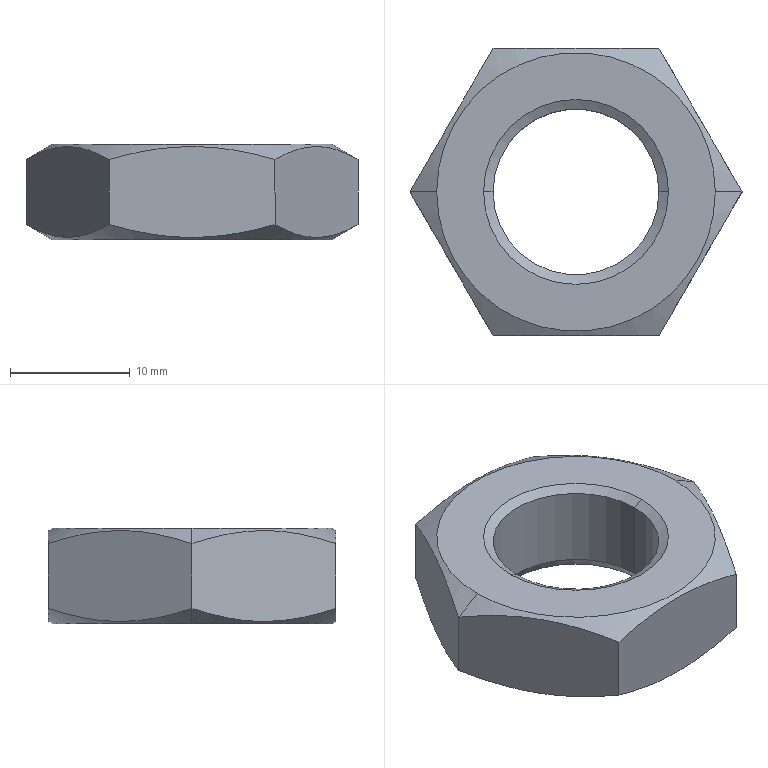Part | SolidWorks | features RevCut 2, Chamfer 1, Extrusion 1, LPattern 1 | 1 solid | 18 faces | box 27.713 x 24 x 8 mm | volume 2715 mm3 | cone 8 | plane 8 | cylinder 2 | commonest cylinder face diameters 13.835 x2
STEP:
#1=CARTESIAN_POINT('',(-6.918,0.,-0.4619));
#2=VERTEX_POINT('',#1);
#3=CARTESIAN_POINT('',(6.918,0.,-0.4619));
#4=VERTEX_POINT('',#3);
#5=CARTESIAN_POINT('',(0.,0.,-0.4619));
#6=DIRECTION('',(0.,0.,1.));
#7=DIRECTION('',(1.,0.,0.));
#8=AXIS2_PLACEMENT_3D('',#5,#6,#7);
#9=CIRCLE('',#8,6.918);
#10=EDGE_CURVE('',#2,#4,#9,.T.);
#11=ORIENTED_EDGE('',*,*,#10,.F.);
#12=CARTESIAN_POINT('',(-7.718,0.,0.));
#13=VERTEX_POINT('',#12);
#14=CARTESIAN_POINT('',(-6.918,0.,-0.4619));
#15=DIRECTION('',(-0.866,0.,0.5));
#16=VECTOR('',#15,1000.);
#17=LINE('',#14,#16);
#18=EDGE_CURVE('',#2,#13,#17,.T.);
#19=ORIENTED_EDGE('',*,*,#18,.T.);
#20=CARTESIAN_POINT('',(7.718,0.,0.));
#21=VERTEX_POINT('',#20);
#22=CARTESIAN_POINT('',(0.,0.,0.));
#23=DIRECTION('',(0.,0.,-1.));
#24=DIRECTION('',(1.,0.,0.));
#25=AXIS2_PLACEMENT_3D('',#22,#23,#24);
#26=CIRCLE('',#25,7.718);
#27=EDGE_CURVE('',#21,#13,#26,.T.);
#28=ORIENTED_EDGE('',*,*,#27,.F.);
#29=CARTESIAN_POINT('',(6.918,0.,-0.4619));
#30=DIRECTION('',(0.866,0.,0.5));
#31=VECTOR('',#30,1000.);
#32=LINE('',#29,#31);
#33=EDGE_CURVE('',#4,#21,#32,.T.);
#34=ORIENTED_EDGE('',*,*,#33,.F.);
#35=EDGE_LOOP('',(#11,#19,#28,#34));
#36=FACE_OUTER_BOUND('',#35,.T.);
#37=CARTESIAN_POINT('',(0.,0.,-0.4619));
#38=DIRECTION('',(0.,0.,1.));
#39=DIRECTION('',(1.,0.,0.));
#40=AXIS2_PLACEMENT_3D('',#37,#38,#39);
#41=CONICAL_SURFACE('',#40,6.918,1.047);
#42=ADVANCED_FACE('',(#36),#41,.F.);
#43=CARTESIAN_POINT('',(6.918,0.,-7.2));
#44=VERTEX_POINT('',#43);
#45=CARTESIAN_POINT('',(-6.918,0.,-7.2));
#46=VERTEX_POINT('',#45);
#47=CARTESIAN_POINT('',(0.,0.,-7.2));
#48=DIRECTION('',(0.,0.,-1.));
#49=DIRECTION('',(1.,0.,0.));
#50=AXIS2_PLACEMENT_3D('',#47,#48,#49);
#51=CIRCLE('',#50,6.918);
#52=EDGE_CURVE('',#44,#46,#51,.T.);
#53=ORIENTED_EDGE('',*,*,#52,.F.);
#54=CARTESIAN_POINT('',(7.379,0.,-8.));
#55=VERTEX_POINT('',#54);
#56=CARTESIAN_POINT('',(7.379,0.,-8.));
#57=DIRECTION('',(0.5,0.,-0.866));
#58=VECTOR('',#57,1000.);
#59=LINE('',#56,#58);
#60=EDGE_CURVE('',#44,#55,#59,.T.);
#61=ORIENTED_EDGE('',*,*,#60,.T.);
#62=CARTESIAN_POINT('',(-7.379,0.,-8.));
#63=VERTEX_POINT('',#62);
#64=CARTESIAN_POINT('',(0.,0.,-8.));
#65=DIRECTION('',(0.,0.,1.));
#66=DIRECTION('',(1.,0.,0.));
#67=AXIS2_PLACEMENT_3D('',#64,#65,#66);
#68=CIRCLE('',#67,7.379);
#69=EDGE_CURVE('',#63,#55,#68,.T.);
#70=ORIENTED_EDGE('',*,*,#69,.F.);
#71=CARTESIAN_POINT('',(-7.379,0.,-8.));
#72=DIRECTION('',(-0.5,0.,-0.866));
#73=VECTOR('',#72,1000.);
#74=LINE('',#71,#73);
#75=EDGE_CURVE('',#46,#63,#74,.T.);
#76=ORIENTED_EDGE('',*,*,#75,.F.);
#77=EDGE_LOOP('',(#53,#61,#70,#76));
#78=FACE_OUTER_BOUND('',#77,.T.);
#79=CARTESIAN_POINT('',(0.,0.,-8.));
#80=DIRECTION('',(0.,0.,-1.));
#81=DIRECTION('',(-1.,0.,0.));
#82=AXIS2_PLACEMENT_3D('',#79,#80,#81);
#83=CONICAL_SURFACE('',#82,7.379,0.5236);
#84=ADVANCED_FACE('',(#78),#83,.F.);
#85=CARTESIAN_POINT('',(-11.625,0.,0.));
#86=VERTEX_POINT('',#85);
#87=CARTESIAN_POINT('',(11.625,0.,0.));
#88=VERTEX_POINT('',#87);
#89=CARTESIAN_POINT('',(0.,0.,0.));
#90=DIRECTION('',(0.,0.,-1.));
#91=DIRECTION('',(-1.,0.,0.));
#92=AXIS2_PLACEMENT_3D('',#89,#90,#91);
#93=CIRCLE('',#92,11.625);
#94=EDGE_CURVE('',#86,#88,#93,.T.);
#95=ORIENTED_EDGE('',*,*,#94,.T.);
#96=CARTESIAN_POINT('',(13.856,0.,-1.288));
#97=VERTEX_POINT('',#96);
#98=CARTESIAN_POINT('',(11.625,0.,0.));
#99=DIRECTION('',(0.866,0.,-0.5));
#100=VECTOR('',#99,1000.);
#101=LINE('',#98,#100);
#102=EDGE_CURVE('',#88,#97,#101,.T.);
#103=ORIENTED_EDGE('',*,*,#102,.T.);
#104=CARTESIAN_POINT('',(6.928,12.,-1.288));
#105=VERTEX_POINT('',#104);
#106=CARTESIAN_POINT('',(13.856,0.,-1.288));
#107=CARTESIAN_POINT('',(13.291,0.9797,-0.9617));
#108=CARTESIAN_POINT('',(12.721,1.967,-0.6926));
#109=CARTESIAN_POINT('',(11.57,3.961,-0.3197));
#110=CARTESIAN_POINT('',(10.988,4.968,-0.2173));
#111=CARTESIAN_POINT('',(10.104,6.499,-0.2161));
#112=CARTESIAN_POINT('',(9.809,7.011,-0.2412));
#113=CARTESIAN_POINT('',(9.223,8.025,-0.3389));
#114=CARTESIAN_POINT('',(8.933,8.528,-0.4114));
#115=CARTESIAN_POINT('',(8.066,10.03,-0.6915));
#116=CARTESIAN_POINT('',(7.495,11.019,-0.9613));
#117=CARTESIAN_POINT('',(6.928,12.,-1.288));
#118=B_SPLINE_CURVE_WITH_KNOTS('',3,(#106,#107,#108,#109,#110,#111,#112,#113,#114,#115,#116,#117),.UNSPECIFIED.,.F.,.F.,(4,2,2,2,2,4),(0.000000238,0.003499,0.006997,0.008747,0.0105,0.01399),.UNSPECIFIED.);
#119=EDGE_CURVE('',#97,#105,#118,.T.);
#120=ORIENTED_EDGE('',*,*,#119,.T.);
#121=CARTESIAN_POINT('',(-6.928,12.,-1.288));
#122=VERTEX_POINT('',#121);
#123=CARTESIAN_POINT('',(6.928,12.,-1.288));
#124=CARTESIAN_POINT('',(5.808,12.,-0.965));
#125=CARTESIAN_POINT('',(4.674,12.,-0.6957));
#126=CARTESIAN_POINT('',(2.938,12.,-0.414));
#127=CARTESIAN_POINT('',(2.353,12.,-0.3404));
#128=CARTESIAN_POINT('',(1.175,12.,-0.2415));
#129=CARTESIAN_POINT('',(0.5876,12.,-0.2166));
#130=CARTESIAN_POINT('',(-1.169,12.,-0.2164));
#131=CARTESIAN_POINT('',(-2.332,12.,-0.317));
#132=CARTESIAN_POINT('',(-4.647,12.,-0.69));
#133=CARTESIAN_POINT('',(-5.801,12.,-0.963));
#134=CARTESIAN_POINT('',(-6.928,12.,-1.288));
#135=B_SPLINE_CURVE_WITH_KNOTS('',3,(#123,#124,#125,#126,#127,#128,#129,#130,#131,#132,#133,#134),.UNSPECIFIED.,.F.,.F.,(4,2,2,2,2,4),(0.005114,0.008611,0.01036,0.01211,0.0156,0.0191),.UNSPECIFIED.);
#136=EDGE_CURVE('',#105,#122,#135,.T.);
#137=ORIENTED_EDGE('',*,*,#136,.T.);
#138=CARTESIAN_POINT('',(-13.856,0.,-1.288));
#139=VERTEX_POINT('',#138);
#140=CARTESIAN_POINT('',(-6.928,12.,-1.288));
#141=CARTESIAN_POINT('',(-7.494,11.02,-0.9617));
#142=CARTESIAN_POINT('',(-8.064,10.033,-0.6926));
#143=CARTESIAN_POINT('',(-9.215,8.039,-0.3197));
#144=CARTESIAN_POINT('',(-9.797,7.032,-0.2173));
#145=CARTESIAN_POINT('',(-10.68,5.501,-0.2161));
#146=CARTESIAN_POINT('',(-10.976,4.989,-0.2412));
#147=CARTESIAN_POINT('',(-11.561,3.975,-0.3389));
#148=CARTESIAN_POINT('',(-11.852,3.472,-0.4114));
#149=CARTESIAN_POINT('',(-12.719,1.97,-0.6915));
#150=CARTESIAN_POINT('',(-13.29,0.9809,-0.9613));
#151=CARTESIAN_POINT('',(-13.856,0.,-1.288));
#152=B_SPLINE_CURVE_WITH_KNOTS('',3,(#140,#141,#142,#143,#144,#145,#146,#147,#148,#149,#150,#151),.UNSPECIFIED.,.F.,.F.,(4,2,2,2,2,4),(0.000000238,0.003499,0.006997,0.008747,0.0105,0.01399),.UNSPECIFIED.);
#153=EDGE_CURVE('',#122,#139,#152,.T.);
#154=ORIENTED_EDGE('',*,*,#153,.T.);
#155=CARTESIAN_POINT('',(-11.625,0.,0.));
#156=DIRECTION('',(-0.866,0.,-0.5));
#157=VECTOR('',#156,1000.);
#158=LINE('',#155,#157);
#159=EDGE_CURVE('',#86,#139,#158,.T.);
#160=ORIENTED_EDGE('',*,*,#159,.F.);
#161=EDGE_LOOP('',(#95,#103,#120,#137,#154,#160));
#162=FACE_OUTER_BOUND('',#161,.T.);
#163=CARTESIAN_POINT('',(0.,0.,0.));
#164=DIRECTION('',(0.,0.,-1.));
#165=DIRECTION('',(-1.,0.,0.));
#166=AXIS2_PLACEMENT_3D('',#163,#164,#165);
#167=CONICAL_SURFACE('',#166,11.625,1.047);
#168=ADVANCED_FACE('',(#162),#167,.T.);
#169=CARTESIAN_POINT('',(-11.625,0.,-8.));
#170=VERTEX_POINT('',#169);
#171=CARTESIAN_POINT('',(11.625,0.,-8.));
#172=VERTEX_POINT('',#171);
#173=CARTESIAN_POINT('',(0.,0.,-8.));
#174=DIRECTION('',(0.,0.,-1.));
#175=DIRECTION('',(-1.,0.,0.));
#176=AXIS2_PLACEMENT_3D('',#173,#174,#175);
#177=CIRCLE('',#176,11.625);
#178=EDGE_CURVE('',#170,#172,#177,.T.);
#179=ORIENTED_EDGE('',*,*,#178,.F.);
#180=CARTESIAN_POINT('',(-13.856,0.,-6.712));
#181=VERTEX_POINT('',#180);
#182=CARTESIAN_POINT('',(-13.856,0.,-6.712));
#183=DIRECTION('',(-0.866,0.,0.5));
#184=VECTOR('',#183,1000.);
#185=LINE('',#182,#184);
#186=EDGE_CURVE('',#170,#181,#185,.T.);
#187=ORIENTED_EDGE('',*,*,#186,.T.);
#188=CARTESIAN_POINT('',(-6.928,12.,-6.712));
#189=VERTEX_POINT('',#188);
#190=CARTESIAN_POINT('',(-13.856,0.,-6.712));
#191=CARTESIAN_POINT('',(-13.291,0.9797,-7.038));
#192=CARTESIAN_POINT('',(-12.721,1.967,-7.307));
#193=CARTESIAN_POINT('',(-11.57,3.961,-7.68));
#194=CARTESIAN_POINT('',(-10.988,4.968,-7.783));
#195=CARTESIAN_POINT('',(-10.104,6.499,-7.784));
#196=CARTESIAN_POINT('',(-9.809,7.011,-7.759));
#197=CARTESIAN_POINT('',(-9.223,8.025,-7.661));
#198=CARTESIAN_POINT('',(-8.933,8.528,-7.589));
#199=CARTESIAN_POINT('',(-8.066,10.03,-7.308));
#200=CARTESIAN_POINT('',(-7.495,11.019,-7.039));
#201=CARTESIAN_POINT('',(-6.928,12.,-6.712));
#202=B_SPLINE_CURVE_WITH_KNOTS('',3,(#190,#191,#192,#193,#194,#195,#196,#197,#198,#199,#200,#201),.UNSPECIFIED.,.F.,.F.,(4,2,2,2,2,4),(0.000000238,0.003499,0.006997,0.008747,0.0105,0.01399),.UNSPECIFIED.);
#203=EDGE_CURVE('',#181,#189,#202,.T.);
#204=ORIENTED_EDGE('',*,*,#203,.T.);
#205=CARTESIAN_POINT('',(6.928,12.,-6.712));
#206=VERTEX_POINT('',#205);
#207=CARTESIAN_POINT('',(-6.928,12.,-6.712));
#208=CARTESIAN_POINT('',(-5.801,12.,-7.037));
#209=CARTESIAN_POINT('',(-4.647,12.,-7.31));
#210=CARTESIAN_POINT('',(-2.332,12.,-7.683));
#211=CARTESIAN_POINT('',(-1.169,12.,-7.784));
#212=CARTESIAN_POINT('',(0.5876,12.,-7.783));
#213=CARTESIAN_POINT('',(1.175,12.,-7.759));
#214=CARTESIAN_POINT('',(2.353,12.,-7.66));
#215=CARTESIAN_POINT('',(2.938,12.,-7.586));
#216=CARTESIAN_POINT('',(4.674,12.,-7.304));
#217=CARTESIAN_POINT('',(5.808,12.,-7.035));
#218=CARTESIAN_POINT('',(6.928,12.,-6.712));
#219=B_SPLINE_CURVE_WITH_KNOTS('',3,(#207,#208,#209,#210,#211,#212,#213,#214,#215,#216,#217,#218),.UNSPECIFIED.,.F.,.F.,(4,2,2,2,2,4),(0.01233,0.01583,0.01934,0.02109,0.02284,0.02635),.UNSPECIFIED.);
#220=EDGE_CURVE('',#189,#206,#219,.T.);
#221=ORIENTED_EDGE('',*,*,#220,.T.);
#222=CARTESIAN_POINT('',(13.856,0.,-6.712));
#223=VERTEX_POINT('',#222);
#224=CARTESIAN_POINT('',(6.928,12.,-6.712));
#225=CARTESIAN_POINT('',(7.494,11.02,-7.038));
#226=CARTESIAN_POINT('',(8.064,10.033,-7.307));
#227=CARTESIAN_POINT('',(9.215,8.039,-7.68));
#228=CARTESIAN_POINT('',(9.797,7.032,-7.783));
#229=CARTESIAN_POINT('',(10.68,5.501,-7.784));
#230=CARTESIAN_POINT('',(10.976,4.989,-7.759));
#231=CARTESIAN_POINT('',(11.561,3.975,-7.661));
#232=CARTESIAN_POINT('',(11.852,3.472,-7.589));
#233=CARTESIAN_POINT('',(12.719,1.97,-7.308));
#234=CARTESIAN_POINT('',(13.29,0.9809,-7.039));
#235=CARTESIAN_POINT('',(13.856,0.,-6.712));
#236=B_SPLINE_CURVE_WITH_KNOTS('',3,(#224,#225,#226,#227,#228,#229,#230,#231,#232,#233,#234,#235),.UNSPECIFIED.,.F.,.F.,(4,2,2,2,2,4),(0.000000238,0.003499,0.006997,0.008747,0.0105,0.01399),.UNSPECIFIED.);
#237=EDGE_CURVE('',#206,#223,#236,.T.);
#238=ORIENTED_EDGE('',*,*,#237,.T.);
#239=CARTESIAN_POINT('',(13.856,0.,-6.712));
#240=DIRECTION('',(0.866,0.,0.5));
#241=VECTOR('',#240,1000.);
#242=LINE('',#239,#241);
#243=EDGE_CURVE('',#172,#223,#242,.T.);
#244=ORIENTED_EDGE('',*,*,#243,.F.);
#245=EDGE_LOOP('',(#179,#187,#204,#221,#238,#244));
#246=FACE_OUTER_BOUND('',#245,.T.);
#247=CARTESIAN_POINT('',(0.,0.,-6.712));
#248=DIRECTION('',(0.,0.,1.));
#249=DIRECTION('',(1.,0.,0.));
#250=AXIS2_PLACEMENT_3D('',#247,#248,#249);
#251=CONICAL_SURFACE('',#250,13.856,1.047);
#252=ADVANCED_FACE('',(#246),#251,.T.);
#253=ORIENTED_EDGE('',*,*,#52,.T.);
#254=CARTESIAN_POINT('',(-6.918,0.,-8.));
#255=DIRECTION('',(0.,0.,1.));
#256=VECTOR('',#255,1000.);
#257=LINE('',#254,#256);
#258=EDGE_CURVE('',#46,#2,#257,.T.);
#259=ORIENTED_EDGE('',*,*,#258,.T.);
#260=ORIENTED_EDGE('',*,*,#10,.T.);
#261=CARTESIAN_POINT('',(6.918,0.,-8.));
#262=DIRECTION('',(0.,0.,1.));
#263=VECTOR('',#262,1000.);
#264=LINE('',#261,#263);
#265=EDGE_CURVE('',#44,#4,#264,.T.);
#266=ORIENTED_EDGE('',*,*,#265,.F.);
#267=EDGE_LOOP('',(#253,#259,#260,#266));
#268=FACE_OUTER_BOUND('',#267,.T.);
#269=CARTESIAN_POINT('',(0.,0.,-8.));
#270=DIRECTION('',(0.,0.,1.));
#271=DIRECTION('',(1.,0.,0.));
#272=AXIS2_PLACEMENT_3D('',#269,#270,#271);
#273=CYLINDRICAL_SURFACE('',#272,6.918);
#274=ADVANCED_FACE('',(#268),#273,.F.);
#275=CARTESIAN_POINT('',(-6.928,-12.,-1.288));
#276=VERTEX_POINT('',#275);
#277=CARTESIAN_POINT('',(6.928,-12.,-1.288));
#278=VERTEX_POINT('',#277);
#279=CARTESIAN_POINT('',(-6.928,-12.,-1.288));
#280=CARTESIAN_POINT('',(-5.801,-12.,-0.963));
#281=CARTESIAN_POINT('',(-4.647,-12.,-0.69));
#282=CARTESIAN_POINT('',(-2.332,-12.,-0.317));
#283=CARTESIAN_POINT('',(-1.169,-12.,-0.2164));
#284=CARTESIAN_POINT('',(0.5876,-12.,-0.2166));
#285=CARTESIAN_POINT('',(1.175,-12.,-0.2415));
#286=CARTESIAN_POINT('',(2.353,-12.,-0.3404));
#287=CARTESIAN_POINT('',(2.938,-12.,-0.414));
#288=CARTESIAN_POINT('',(4.674,-12.,-0.6957));
#289=CARTESIAN_POINT('',(5.808,-12.,-0.965));
#290=CARTESIAN_POINT('',(6.928,-12.,-1.288));
#291=B_SPLINE_CURVE_WITH_KNOTS('',3,(#279,#280,#281,#282,#283,#284,#285,#286,#287,#288,#289,#290),.UNSPECIFIED.,.F.,.F.,(4,2,2,2,2,4),(0.01233,0.01583,0.01934,0.02109,0.02284,0.02635),.UNSPECIFIED.);
#292=EDGE_CURVE('',#276,#278,#291,.T.);
#293=ORIENTED_EDGE('',*,*,#292,.F.);
#294=CARTESIAN_POINT('',(-6.928,-12.,-6.712));
#295=VERTEX_POINT('',#294);
#296=CARTESIAN_POINT('',(-6.928,-12.,-8.));
#297=DIRECTION('',(0.,0.,1.));
#298=VECTOR('',#297,1000.);
#299=LINE('',#296,#298);
#300=EDGE_CURVE('',#295,#276,#299,.T.);
#301=ORIENTED_EDGE('',*,*,#300,.F.);
#302=CARTESIAN_POINT('',(6.928,-12.,-6.712));
#303=VERTEX_POINT('',#302);
#304=CARTESIAN_POINT('',(6.928,-12.,-6.712));
#305=CARTESIAN_POINT('',(5.808,-12.,-7.035));
#306=CARTESIAN_POINT('',(4.674,-12.,-7.304));
#307=CARTESIAN_POINT('',(2.938,-12.,-7.586));
#308=CARTESIAN_POINT('',(2.353,-12.,-7.66));
#309=CARTESIAN_POINT('',(1.175,-12.,-7.759));
#310=CARTESIAN_POINT('',(0.5876,-12.,-7.783));
#311=CARTESIAN_POINT('',(-1.169,-12.,-7.784));
#312=CARTESIAN_POINT('',(-2.332,-12.,-7.683));
#313=CARTESIAN_POINT('',(-4.647,-12.,-7.31));
#314=CARTESIAN_POINT('',(-5.801,-12.,-7.037));
#315=CARTESIAN_POINT('',(-6.928,-12.,-6.712));
#316=B_SPLINE_CURVE_WITH_KNOTS('',3,(#304,#305,#306,#307,#308,#309,#310,#311,#312,#313,#314,#315),.UNSPECIFIED.,.F.,.F.,(4,2,2,2,2,4),(0.005114,0.008611,0.01036,0.01211,0.0156,0.0191),.UNSPECIFIED.);
#317=EDGE_CURVE('',#303,#295,#316,.T.);
#318=ORIENTED_EDGE('',*,*,#317,.F.);
#319=CARTESIAN_POINT('',(6.928,-12.,-8.));
#320=DIRECTION('',(0.,0.,1.));
#321=VECTOR('',#320,1000.);
#322=LINE('',#319,#321);
#323=EDGE_CURVE('',#303,#278,#322,.T.);
#324=ORIENTED_EDGE('',*,*,#323,.T.);
#325=EDGE_LOOP('',(#293,#301,#318,#324));
#326=FACE_OUTER_BOUND('',#325,.T.);
#327=CARTESIAN_POINT('',(-6.928,-12.,-8.));
#328=DIRECTION('',(0.,-1.,0.));
#329=DIRECTION('',(0.,0.,-1.));
#330=AXIS2_PLACEMENT_3D('',#327,#328,#329);
#331=PLANE('',#330);
#332=ADVANCED_FACE('',(#326),#331,.T.);
#333=CARTESIAN_POINT('',(-13.856,0.,-1.288));
#334=CARTESIAN_POINT('',(-13.291,-0.9797,-0.9617));
#335=CARTESIAN_POINT('',(-12.721,-1.967,-0.6926));
#336=CARTESIAN_POINT('',(-11.57,-3.961,-0.3197));
#337=CARTESIAN_POINT('',(-10.988,-4.968,-0.2173));
#338=CARTESIAN_POINT('',(-10.104,-6.499,-0.2161));
#339=CARTESIAN_POINT('',(-9.809,-7.011,-0.2412));
#340=CARTESIAN_POINT('',(-9.223,-8.025,-0.3389));
#341=CARTESIAN_POINT('',(-8.933,-8.528,-0.4114));
#342=CARTESIAN_POINT('',(-8.066,-10.03,-0.6915));
#343=CARTESIAN_POINT('',(-7.495,-11.019,-0.9613));
#344=CARTESIAN_POINT('',(-6.928,-12.,-1.288));
#345=B_SPLINE_CURVE_WITH_KNOTS('',3,(#333,#334,#335,#336,#337,#338,#339,#340,#341,#342,#343,#344),.UNSPECIFIED.,.F.,.F.,(4,2,2,2,2,4),(0.000000238,0.003499,0.006997,0.008747,0.0105,0.01399),.UNSPECIFIED.);
#346=EDGE_CURVE('',#139,#276,#345,.T.);
#347=ORIENTED_EDGE('',*,*,#346,.F.);
#348=CARTESIAN_POINT('',(-13.856,0.,-8.));
#349=DIRECTION('',(0.,0.,1.));
#350=VECTOR('',#349,1000.);
#351=LINE('',#348,#350);
#352=EDGE_CURVE('',#181,#139,#351,.T.);
#353=ORIENTED_EDGE('',*,*,#352,.F.);
#354=CARTESIAN_POINT('',(-6.928,-12.,-6.712));
#355=CARTESIAN_POINT('',(-7.494,-11.02,-7.038));
#356=CARTESIAN_POINT('',(-8.064,-10.033,-7.307));
#357=CARTESIAN_POINT('',(-9.215,-8.039,-7.68));
#358=CARTESIAN_POINT('',(-9.797,-7.032,-7.783));
#359=CARTESIAN_POINT('',(-10.68,-5.501,-7.784));
#360=CARTESIAN_POINT('',(-10.976,-4.989,-7.759));
#361=CARTESIAN_POINT('',(-11.561,-3.975,-7.661));
#362=CARTESIAN_POINT('',(-11.852,-3.472,-7.589));
#363=CARTESIAN_POINT('',(-12.719,-1.97,-7.308));
#364=CARTESIAN_POINT('',(-13.29,-0.9809,-7.039));
#365=CARTESIAN_POINT('',(-13.856,0.,-6.712));
#366=B_SPLINE_CURVE_WITH_KNOTS('',3,(#354,#355,#356,#357,#358,#359,#360,#361,#362,#363,#364,#365),.UNSPECIFIED.,.F.,.F.,(4,2,2,2,2,4),(0.000000238,0.003499,0.006997,0.008747,0.0105,0.01399),.UNSPECIFIED.);
#367=EDGE_CURVE('',#295,#181,#366,.T.);
#368=ORIENTED_EDGE('',*,*,#367,.F.);
#369=ORIENTED_EDGE('',*,*,#300,.T.);
#370=EDGE_LOOP('',(#347,#353,#368,#369));
#371=FACE_OUTER_BOUND('',#370,.T.);
#372=CARTESIAN_POINT('',(-13.856,0.,-8.));
#373=DIRECTION('',(-0.866,-0.5,0.));
#374=DIRECTION('',(0.5,-0.866,0.));
#375=AXIS2_PLACEMENT_3D('',#372,#373,#374);
#376=PLANE('',#375);
#377=ADVANCED_FACE('',(#371),#376,.T.);
#378=ORIENTED_EDGE('',*,*,#153,.F.);
#379=CARTESIAN_POINT('',(-6.928,12.,-8.));
#380=DIRECTION('',(0.,0.,1.));
#381=VECTOR('',#380,1000.);
#382=LINE('',#379,#381);
#383=EDGE_CURVE('',#189,#122,#382,.T.);
#384=ORIENTED_EDGE('',*,*,#383,.F.);
#385=ORIENTED_EDGE('',*,*,#203,.F.);
#386=ORIENTED_EDGE('',*,*,#352,.T.);
#387=EDGE_LOOP('',(#378,#384,#385,#386));
#388=FACE_OUTER_BOUND('',#387,.T.);
#389=CARTESIAN_POINT('',(-6.928,12.,-8.));
#390=DIRECTION('',(-0.866,0.5,0.));
#391=DIRECTION('',(-0.5,-0.866,0.));
#392=AXIS2_PLACEMENT_3D('',#389,#390,#391);
#393=PLANE('',#392);
#394=ADVANCED_FACE('',(#388),#393,.T.);
#395=ORIENTED_EDGE('',*,*,#136,.F.);
#396=CARTESIAN_POINT('',(6.928,12.,-8.));
#397=DIRECTION('',(0.,0.,1.));
#398=VECTOR('',#397,1000.);
#399=LINE('',#396,#398);
#400=EDGE_CURVE('',#206,#105,#399,.T.);
#401=ORIENTED_EDGE('',*,*,#400,.F.);
#402=ORIENTED_EDGE('',*,*,#220,.F.);
#403=ORIENTED_EDGE('',*,*,#383,.T.);
#404=EDGE_LOOP('',(#395,#401,#402,#403));
#405=FACE_OUTER_BOUND('',#404,.T.);
#406=CARTESIAN_POINT('',(6.928,12.,-8.));
#407=DIRECTION('',(0.,1.,0.));
#408=DIRECTION('',(0.,0.,1.));
#409=AXIS2_PLACEMENT_3D('',#406,#407,#408);
#410=PLANE('',#409);
#411=ADVANCED_FACE('',(#405),#410,.T.);
#412=ORIENTED_EDGE('',*,*,#119,.F.);
#413=CARTESIAN_POINT('',(13.856,0.,-8.));
#414=DIRECTION('',(0.,0.,1.));
#415=VECTOR('',#414,1000.);
#416=LINE('',#413,#415);
#417=EDGE_CURVE('',#223,#97,#416,.T.);
#418=ORIENTED_EDGE('',*,*,#417,.F.);
#419=ORIENTED_EDGE('',*,*,#237,.F.);
#420=ORIENTED_EDGE('',*,*,#400,.T.);
#421=EDGE_LOOP('',(#412,#418,#419,#420));
#422=FACE_OUTER_BOUND('',#421,.T.);
#423=CARTESIAN_POINT('',(13.856,0.,-8.));
#424=DIRECTION('',(0.866,0.5,0.));
#425=DIRECTION('',(-0.5,0.866,0.));
#426=AXIS2_PLACEMENT_3D('',#423,#424,#425);
#427=PLANE('',#426);
#428=ADVANCED_FACE('',(#422),#427,.T.);
#429=CARTESIAN_POINT('',(6.928,-12.,-1.288));
#430=CARTESIAN_POINT('',(7.494,-11.02,-0.9617));
#431=CARTESIAN_POINT('',(8.064,-10.033,-0.6926));
#432=CARTESIAN_POINT('',(9.215,-8.039,-0.3197));
#433=CARTESIAN_POINT('',(9.797,-7.032,-0.2173));
#434=CARTESIAN_POINT('',(10.68,-5.501,-0.2161));
#435=CARTESIAN_POINT('',(10.976,-4.989,-0.2412));
#436=CARTESIAN_POINT('',(11.561,-3.975,-0.3389));
#437=CARTESIAN_POINT('',(11.852,-3.472,-0.4114));
#438=CARTESIAN_POINT('',(12.719,-1.97,-0.6915));
#439=CARTESIAN_POINT('',(13.29,-0.9809,-0.9613));
#440=CARTESIAN_POINT('',(13.856,0.,-1.288));
#441=B_SPLINE_CURVE_WITH_KNOTS('',3,(#429,#430,#431,#432,#433,#434,#435,#436,#437,#438,#439,#440),.UNSPECIFIED.,.F.,.F.,(4,2,2,2,2,4),(0.000000238,0.003499,0.006997,0.008747,0.0105,0.01399),.UNSPECIFIED.);
#442=EDGE_CURVE('',#278,#97,#441,.T.);
#443=ORIENTED_EDGE('',*,*,#442,.F.);
#444=ORIENTED_EDGE('',*,*,#323,.F.);
#445=CARTESIAN_POINT('',(13.856,0.,-6.712));
#446=CARTESIAN_POINT('',(13.291,-0.9797,-7.038));
#447=CARTESIAN_POINT('',(12.721,-1.967,-7.307));
#448=CARTESIAN_POINT('',(11.57,-3.961,-7.68));
#449=CARTESIAN_POINT('',(10.988,-4.968,-7.783));
#450=CARTESIAN_POINT('',(10.104,-6.499,-7.784));
#451=CARTESIAN_POINT('',(9.809,-7.011,-7.759));
#452=CARTESIAN_POINT('',(9.223,-8.025,-7.661));
#453=CARTESIAN_POINT('',(8.933,-8.528,-7.589));
#454=CARTESIAN_POINT('',(8.066,-10.03,-7.308));
#455=CARTESIAN_POINT('',(7.495,-11.019,-7.039));
#456=CARTESIAN_POINT('',(6.928,-12.,-6.712));
#457=B_SPLINE_CURVE_WITH_KNOTS('',3,(#445,#446,#447,#448,#449,#450,#451,#452,#453,#454,#455,#456),.UNSPECIFIED.,.F.,.F.,(4,2,2,2,2,4),(0.000000238,0.003499,0.006997,0.008747,0.0105,0.01399),.UNSPECIFIED.);
#458=EDGE_CURVE('',#223,#303,#457,.T.);
#459=ORIENTED_EDGE('',*,*,#458,.F.);
#460=ORIENTED_EDGE('',*,*,#417,.T.);
#461=EDGE_LOOP('',(#443,#444,#459,#460));
#462=FACE_OUTER_BOUND('',#461,.T.);
#463=CARTESIAN_POINT('',(6.928,-12.,-8.));
#464=DIRECTION('',(0.866,-0.5,0.));
#465=DIRECTION('',(0.5,0.866,0.));
#466=AXIS2_PLACEMENT_3D('',#463,#464,#465);
#467=PLANE('',#466);
#468=ADVANCED_FACE('',(#462),#467,.T.);
#469=ORIENTED_EDGE('',*,*,#69,.T.);
#470=CARTESIAN_POINT('',(0.,0.,-8.));
#471=DIRECTION('',(0.,0.,1.));
#472=DIRECTION('',(1.,0.,0.));
#473=AXIS2_PLACEMENT_3D('',#470,#471,#472);
#474=CIRCLE('',#473,7.379);
#475=EDGE_CURVE('',#55,#63,#474,.T.);
#476=ORIENTED_EDGE('',*,*,#475,.T.);
#477=EDGE_LOOP('',(#469,#476));
#478=FACE_BOUND('',#477,.T.);
#479=CARTESIAN_POINT('',(0.,0.,-8.));
#480=DIRECTION('',(0.,0.,-1.));
#481=DIRECTION('',(-1.,0.,0.));
#482=AXIS2_PLACEMENT_3D('',#479,#480,#481);
#483=CIRCLE('',#482,11.625);
#484=EDGE_CURVE('',#172,#170,#483,.T.);
#485=ORIENTED_EDGE('',*,*,#484,.T.);
#486=ORIENTED_EDGE('',*,*,#178,.T.);
#487=EDGE_LOOP('',(#485,#486));
#488=FACE_OUTER_BOUND('',#487,.T.);
#489=CARTESIAN_POINT('',(6.928,-12.,-8.));
#490=DIRECTION('',(0.,0.,1.));
#491=DIRECTION('',(1.,0.,0.));
#492=AXIS2_PLACEMENT_3D('',#489,#490,#491);
#493=PLANE('',#492);
#494=ADVANCED_FACE('',(#478,#488),#493,.F.);
#495=ORIENTED_EDGE('',*,*,#27,.T.);
#496=CARTESIAN_POINT('',(0.,0.,0.));
#497=DIRECTION('',(0.,0.,-1.));
#498=DIRECTION('',(1.,0.,0.));
#499=AXIS2_PLACEMENT_3D('',#496,#497,#498);
#500=CIRCLE('',#499,7.718);
#501=EDGE_CURVE('',#13,#21,#500,.T.);
#502=ORIENTED_EDGE('',*,*,#501,.T.);
#503=EDGE_LOOP('',(#495,#502));
#504=FACE_BOUND('',#503,.T.);
#505=ORIENTED_EDGE('',*,*,#94,.F.);
#506=CARTESIAN_POINT('',(0.,0.,0.));
#507=DIRECTION('',(0.,0.,-1.));
#508=DIRECTION('',(-1.,0.,0.));
#509=AXIS2_PLACEMENT_3D('',#506,#507,#508);
#510=CIRCLE('',#509,11.625);
#511=EDGE_CURVE('',#88,#86,#510,.T.);
#512=ORIENTED_EDGE('',*,*,#511,.F.);
#513=EDGE_LOOP('',(#505,#512));
#514=FACE_OUTER_BOUND('',#513,.T.);
#515=CARTESIAN_POINT('',(6.928,-12.,0.));
#516=DIRECTION('',(0.,0.,1.));
#517=DIRECTION('',(1.,0.,0.));
#518=AXIS2_PLACEMENT_3D('',#515,#516,#517);
#519=PLANE('',#518);
#520=ADVANCED_FACE('',(#504,#514),#519,.T.);
#521=ORIENTED_EDGE('',*,*,#258,.F.);
#522=CARTESIAN_POINT('',(0.,0.,-7.2));
#523=DIRECTION('',(0.,0.,-1.));
#524=DIRECTION('',(1.,0.,0.));
#525=AXIS2_PLACEMENT_3D('',#522,#523,#524);
#526=CIRCLE('',#525,6.918);
#527=EDGE_CURVE('',#46,#44,#526,.T.);
#528=ORIENTED_EDGE('',*,*,#527,.T.);
#529=ORIENTED_EDGE('',*,*,#265,.T.);
#530=CARTESIAN_POINT('',(0.,0.,-0.4619));
#531=DIRECTION('',(0.,0.,1.));
#532=DIRECTION('',(1.,0.,0.));
#533=AXIS2_PLACEMENT_3D('',#530,#531,#532);
#534=CIRCLE('',#533,6.918);
#535=EDGE_CURVE('',#4,#2,#534,.T.);
#536=ORIENTED_EDGE('',*,*,#535,.T.);
#537=EDGE_LOOP('',(#521,#528,#529,#536));
#538=FACE_OUTER_BOUND('',#537,.T.);
#539=CARTESIAN_POINT('',(0.,0.,-8.));
#540=DIRECTION('',(0.,0.,1.));
#541=DIRECTION('',(1.,0.,0.));
#542=AXIS2_PLACEMENT_3D('',#539,#540,#541);
#543=CYLINDRICAL_SURFACE('',#542,6.918);
#544=ADVANCED_FACE('',(#538),#543,.F.);
#545=ORIENTED_EDGE('',*,*,#186,.F.);
#546=ORIENTED_EDGE('',*,*,#484,.F.);
#547=ORIENTED_EDGE('',*,*,#243,.T.);
#548=ORIENTED_EDGE('',*,*,#458,.T.);
#549=ORIENTED_EDGE('',*,*,#317,.T.);
#550=ORIENTED_EDGE('',*,*,#367,.T.);
#551=EDGE_LOOP('',(#545,#546,#547,#548,#549,#550));
#552=FACE_OUTER_BOUND('',#551,.T.);
#553=CARTESIAN_POINT('',(0.,0.,-6.712));
#554=DIRECTION('',(0.,0.,1.));
#555=DIRECTION('',(1.,0.,0.));
#556=AXIS2_PLACEMENT_3D('',#553,#554,#555);
#557=CONICAL_SURFACE('',#556,13.856,1.047);
#558=ADVANCED_FACE('',(#552),#557,.T.);
#559=ORIENTED_EDGE('',*,*,#102,.F.);
#560=ORIENTED_EDGE('',*,*,#511,.T.);
#561=ORIENTED_EDGE('',*,*,#159,.T.);
#562=ORIENTED_EDGE('',*,*,#346,.T.);
#563=ORIENTED_EDGE('',*,*,#292,.T.);
#564=ORIENTED_EDGE('',*,*,#442,.T.);
#565=EDGE_LOOP('',(#559,#560,#561,#562,#563,#564));
#566=FACE_OUTER_BOUND('',#565,.T.);
#567=CARTESIAN_POINT('',(0.,0.,0.));
#568=DIRECTION('',(0.,0.,-1.));
#569=DIRECTION('',(-1.,0.,0.));
#570=AXIS2_PLACEMENT_3D('',#567,#568,#569);
#571=CONICAL_SURFACE('',#570,11.625,1.047);
#572=ADVANCED_FACE('',(#566),#571,.T.);
#573=ORIENTED_EDGE('',*,*,#60,.F.);
#574=ORIENTED_EDGE('',*,*,#527,.F.);
#575=ORIENTED_EDGE('',*,*,#75,.T.);
#576=ORIENTED_EDGE('',*,*,#475,.F.);
#577=EDGE_LOOP('',(#573,#574,#575,#576));
#578=FACE_OUTER_BOUND('',#577,.T.);
#579=CARTESIAN_POINT('',(0.,0.,-8.));
#580=DIRECTION('',(0.,0.,-1.));
#581=DIRECTION('',(-1.,0.,0.));
#582=AXIS2_PLACEMENT_3D('',#579,#580,#581);
#583=CONICAL_SURFACE('',#582,7.379,0.5236);
#584=ADVANCED_FACE('',(#578),#583,.F.);
#585=ORIENTED_EDGE('',*,*,#18,.F.);
#586=ORIENTED_EDGE('',*,*,#535,.F.);
#587=ORIENTED_EDGE('',*,*,#33,.T.);
#588=ORIENTED_EDGE('',*,*,#501,.F.);
#589=EDGE_LOOP('',(#585,#586,#587,#588));
#590=FACE_OUTER_BOUND('',#589,.T.);
#591=CARTESIAN_POINT('',(0.,0.,-0.4619));
#592=DIRECTION('',(0.,0.,1.));
#593=DIRECTION('',(1.,0.,0.));
#594=AXIS2_PLACEMENT_3D('',#591,#592,#593);
#595=CONICAL_SURFACE('',#594,6.918,1.047);
#596=ADVANCED_FACE('',(#590),#595,.F.);
#597=CLOSED_SHELL('',(#42,#84,#168,#252,#274,#332,#377,#394,#411,#428,#468,#494,#520,#544,#558,#572,#584,#596));
#598=MANIFOLD_SOLID_BREP('',#597);
#599=CARTESIAN_POINT('',(0.,0.,0.));
#600=DIRECTION('',(0.,0.,1.));
#601=DIRECTION('',(1.,0.,0.));
#602=AXIS2_PLACEMENT_3D('',#599,#600,#601);
#603=(LENGTH_UNIT()NAMED_UNIT(*)SI_UNIT(.MILLI.,.METRE.));
#604=UNCERTAINTY_MEASURE_WITH_UNIT(LENGTH_MEASURE(0.00001),#603,'','');
#605=(NAMED_UNIT(*)PLANE_ANGLE_UNIT()SI_UNIT($,.RADIAN.));
#606=(NAMED_UNIT(*)SI_UNIT($,.STERADIAN.)SOLID_ANGLE_UNIT());
#607=(GEOMETRIC_REPRESENTATION_CONTEXT(3)GLOBAL_UNCERTAINTY_ASSIGNED_CONTEXT((#604))GLOBAL_UNIT_ASSIGNED_CONTEXT((#603,#605,#606))REPRESENTATION_CONTEXT('',''));
#608=ADVANCED_BREP_SHAPE_REPRESENTATION('',(#598,#602),#607);